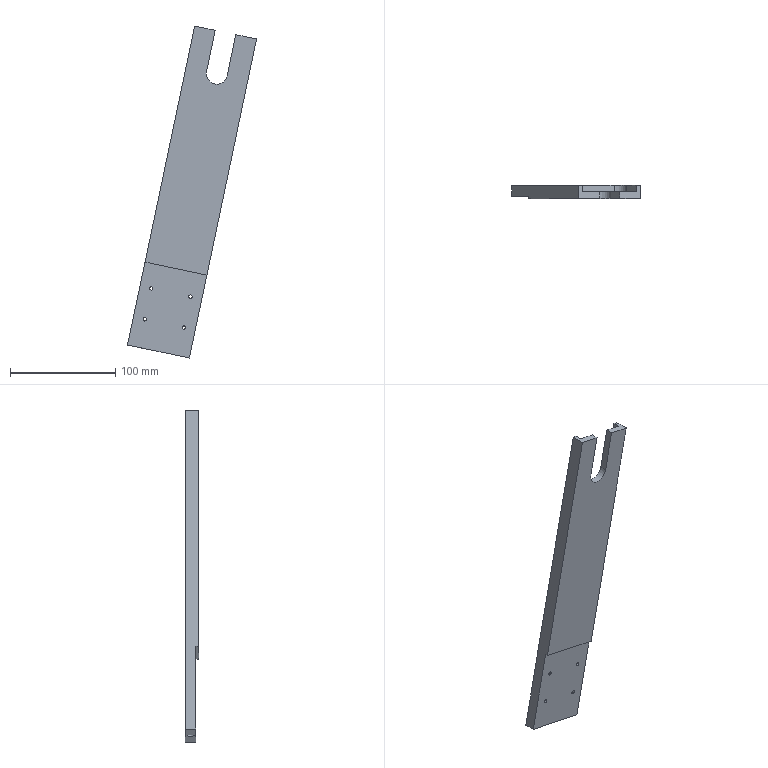Part | STEP file | SN10_006_004_GAVETA | 1 solid | 24 faces | box 122.344 x 12.5 x 315.126 mm | volume 195820 mm3 | plane 15 | cylinder 8 | cone 1 | commonest cylinder face diameters 3.242 x4 20 x3 6.647 x1